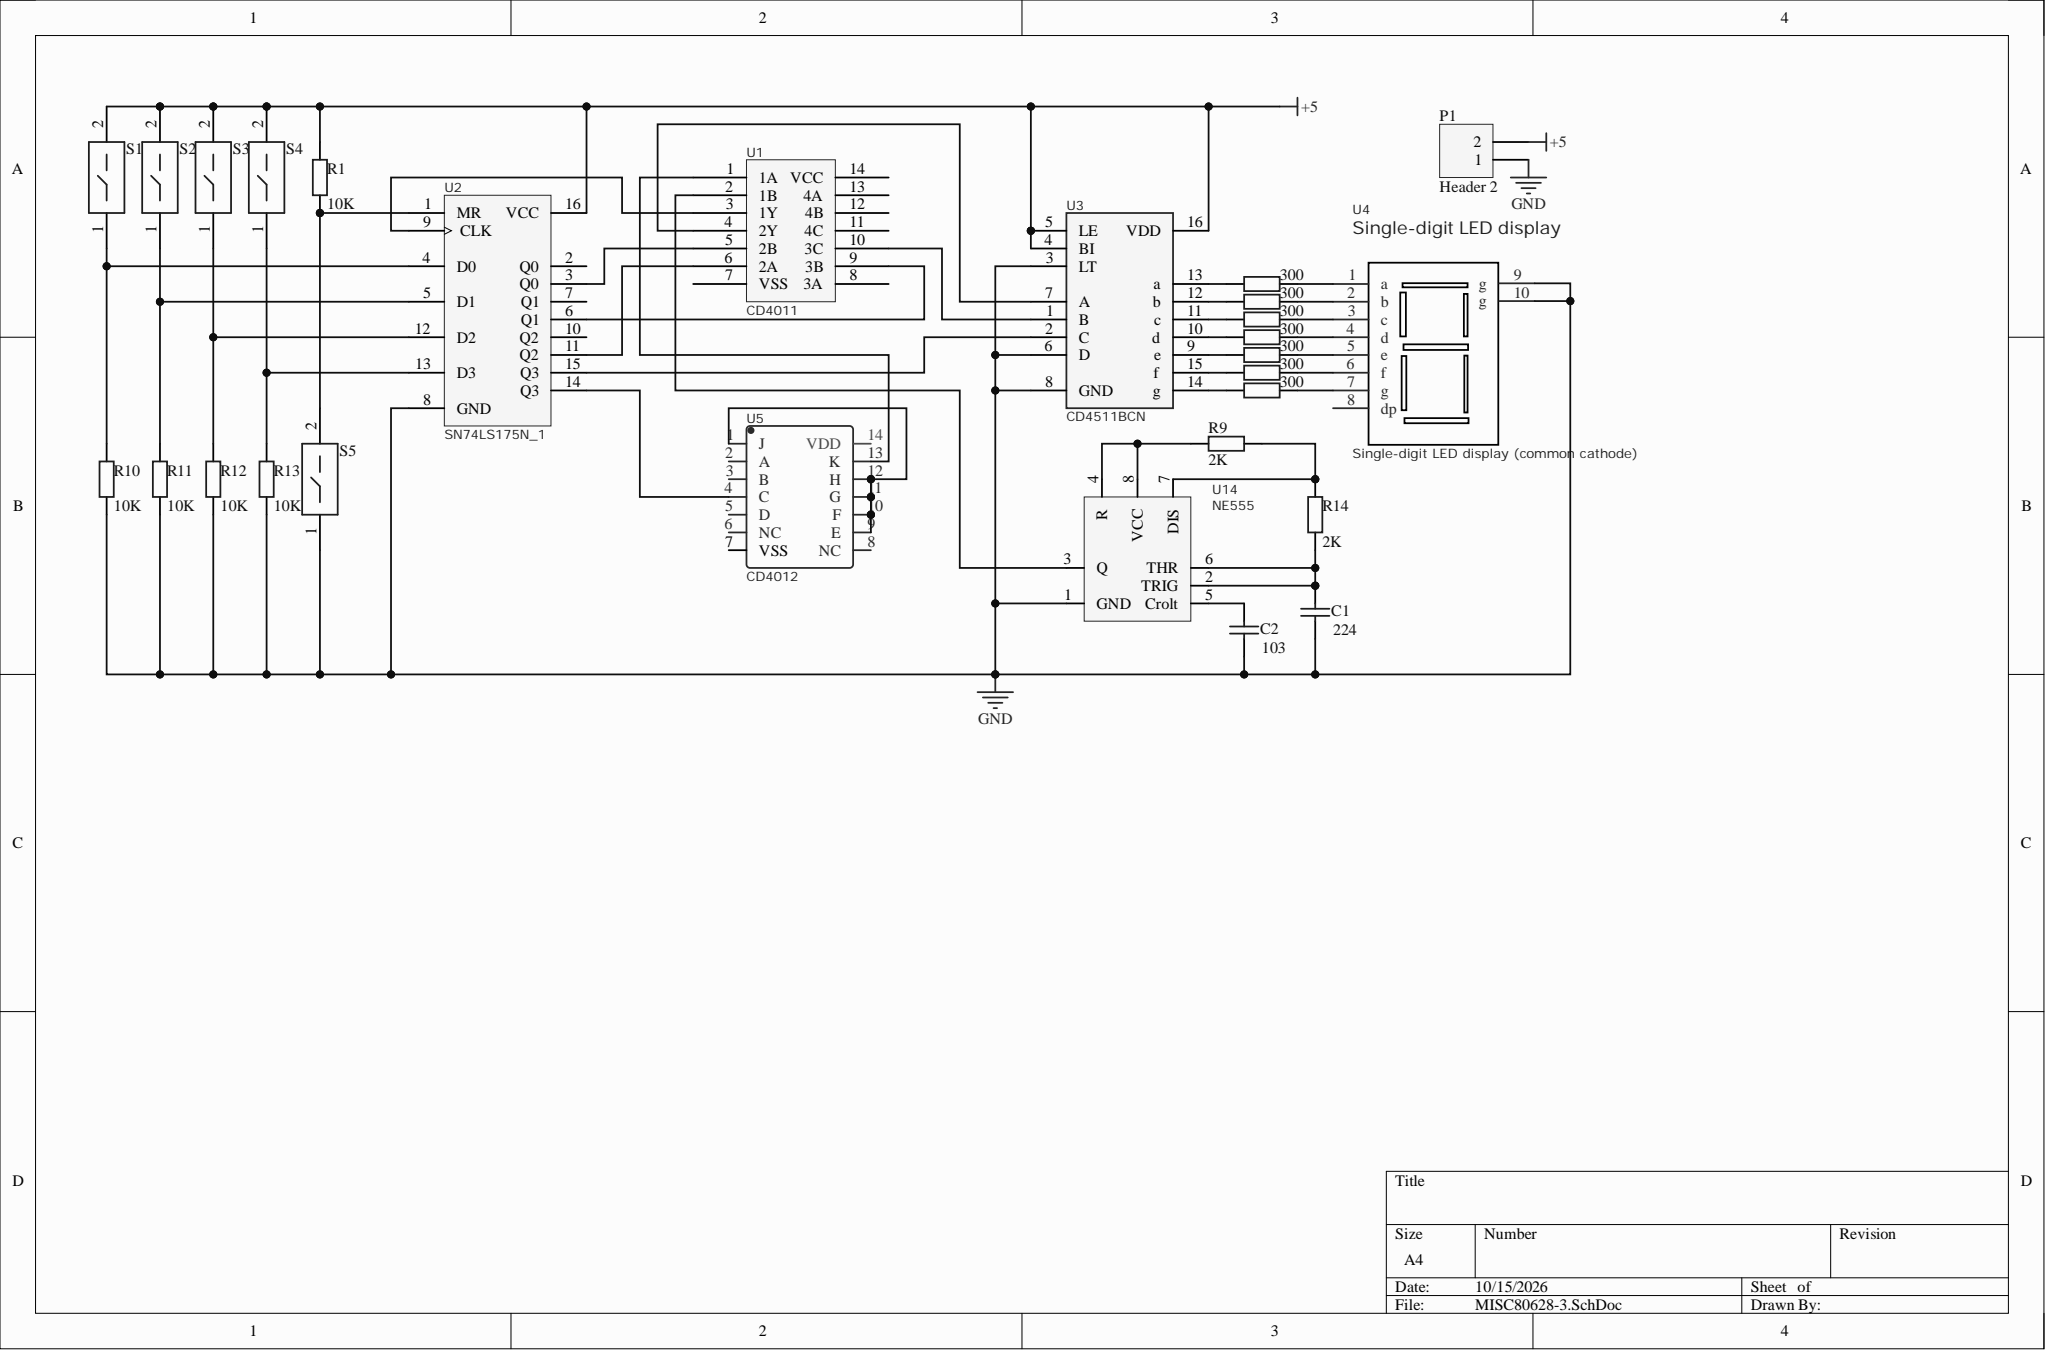Circuit board | Altium Designer | 28 parts | 36 nets
Bill of materials:
Comment,Description,Designator,Footprint,LibRef,Quantity
"Cap","Capacitor","C1, C2","RAD-0.3","Cap","2"
"Header 2","Header, 2-Pin","P1","HDR1X2","Header 2","1"
"Res2","Resistor","R1, R2, R3, R4, R5, R6, R7, R8, R9, R10, R11, R12, R13, R14","AXIAL-0.4","Res2","14"
"SW1-DIP2","","S1, S2, S3, S4, S5","DIP-1P","SW1-DIP2","5"
"CD4011","","U1","CD4011","CD4011","1"
"SN74LS175N_1","","U2","N016","SN74LS175N_1","1"
"CD4511BCN","","U3","CD4511BCN","CD4511BCN","1"
"Single-digit LED display (common cathode)","","U4","PCBComponent_1","一位数码管（共阴极）","1"
"CD4012","","U5","DIP14","CD4012BM","1"
"NE555","","U14","DIP-8-NE555","NE555 (2)","1"
Netlist (Protel format):
[
C1
RAD-0.3
Cap



]
[
C2
RAD-0.3
Cap



]
[
P1
HDR1X2
Header 2



]
[
R1
AXIAL-0.4
Res2



]
[
R2
AXIAL-0.4
Res2



]
[
R3
AXIAL-0.4
Res2



]
[
R4
AXIAL-0.4
Res2



]
[
R5
AXIAL-0.4
Res2



]
[
R6
AXIAL-0.4
Res2



]
[
R7
AXIAL-0.4
Res2



]
[
R8
AXIAL-0.4
Res2



]
[
R9
AXIAL-0.4
Res2



]
[
R10
AXIAL-0.4
Res2



]
[
R11
AXIAL-0.4
Res2



]
[
R12
AXIAL-0.4
Res2



]
[
R13
AXIAL-0.4
Res2



]
[
R14
AXIAL-0.4
Res2



]
[
S1
DIP-1P
SW1-DIP2



]
[
S2
DIP-1P
SW1-DIP2



]
[
S3
DIP-1P
SW1-DIP2



]
[
S4
DIP-1P
SW1-DIP2



]
[
S5
DIP-1P
SW1-DIP2



]
[
U1
CD4011
CD4011



]
[
U2
N016
SN74LS175N_1



]
[
U3
CD4511BCN
CD4511BCN



]
[
U4
PCBComponent_1
Single-digit LED display (common cathode)



]
[
U5
DIP14
CD4012



]
[
U14
DIP-8-NE555
NE555



]
(
NetU5_1
U5-1
U5-9
U5-10
U5-11
U5-12
)
(
NetU2_15
U2-15
U3-2
)
(
NetU2_14
U2-14
U5-4
)
(
NetU1_10
U1-10
U3-1
)
(
NetU1_9
U1-9
U2-6
)
(
NetU1_6
U1-6
U2-11
)
(
NetU1_5
U1-5
U2-3
)
(
NetU1_4
U1-4
U3-7
)
(
NetU1_3
U1-3
U2-9
)
(
NetU1_2
U1-2
U14-3
)
(
NetU1_1
U1-1
U5-13
)
(
NetR13_2
R13-2
S4-1
U2-13
)
(
NetR12_2
R12-2
S3-1
U2-12
)
(
NetR11_2
R11-2
S2-1
U2-5
)
(
NetR10_2
R10-2
S1-1
U2-4
)
(
NetR9_2
R9-2
U14-4
U14-8
)
(
NetR9_1
R9-1
R14-2
U14-7
)
(
NetR8_2
R8-2
U3-14
)
(
NetR8_1
R8-1
U4-7
)
(
NetR7_2
R7-2
U3-15
)
(
NetR7_1
R7-1
U4-6
)
(
NetR6_2
R6-2
U3-9
)
(
NetR6_1
R6-1
U4-5
)
(
NetR5_2
R5-2
U3-10
)
(
NetR5_1
R5-1
U4-4
)
(
NetR4_2
R4-2
U3-11
)
(
NetR4_1
R4-1
U4-3
)
(
NetR3_2
R3-2
U3-12
)
(
NetR3_1
R3-1
U4-2
)
(
NetR2_2
R2-2
U3-13
)
(
NetR2_1
R2-1
U4-1
)
(
NetR1_1
R1-1
S5-2
U2-1
)
(
NetC2_2
C2-2
U14-5
)
(
NetC1_2
C1-2
R14-1
U14-2
U14-6
)
(
GND
C1-1
C2-1
P1-1
R10-1
R11-1
R12-1
R13-1
S5-1
U2-8
U3-3
U3-6
U3-8
U4-9
U4-10
U14-1
)
(
+5
P1-2
R1-2
S1-2
S2-2
S3-2
S4-2
U2-16
U3-4
U3-5
U3-16
)